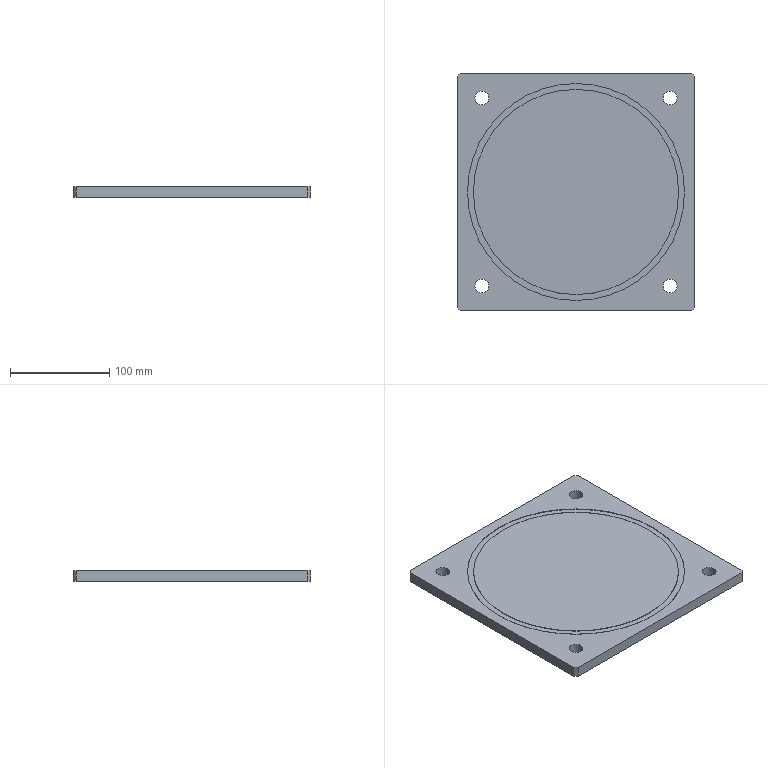Part | SolidWorks | features ICE 2, Chamfer 1, Extrusion 1 | 1 solid | 24 faces | box 240 x 240 x 11 mm | volume 624621 mm3 | cylinder 12 | plane 12 | commonest cylinder face diameters 14 x8 207 x2 219 x2
STEP:
#1=CARTESIAN_POINT('',(-88.,-95.,0.));
#2=VERTEX_POINT('',#1);
#3=CARTESIAN_POINT('',(-102.,-95.,0.));
#4=VERTEX_POINT('',#3);
#5=CARTESIAN_POINT('',(-95.,-95.,0.));
#6=DIRECTION('',(0.,0.,-1.));
#7=DIRECTION('',(-1.,0.,0.));
#8=AXIS2_PLACEMENT_3D('',#5,#6,#7);
#9=CIRCLE('',#8,7.);
#10=EDGE_CURVE('',#2,#4,#9,.T.);
#11=ORIENTED_EDGE('',*,*,#10,.T.);
#12=CARTESIAN_POINT('',(-102.,-95.,11.));
#13=VERTEX_POINT('',#12);
#14=CARTESIAN_POINT('',(-102.,-95.,-48.));
#15=DIRECTION('',(0.,0.,1.));
#16=VECTOR('',#15,1000.);
#17=LINE('',#14,#16);
#18=EDGE_CURVE('',#4,#13,#17,.T.);
#19=ORIENTED_EDGE('',*,*,#18,.T.);
#20=CARTESIAN_POINT('',(-88.,-95.,11.));
#21=VERTEX_POINT('',#20);
#22=CARTESIAN_POINT('',(-95.,-95.,11.));
#23=DIRECTION('',(0.,0.,1.));
#24=DIRECTION('',(1.,0.,0.));
#25=AXIS2_PLACEMENT_3D('',#22,#23,#24);
#26=CIRCLE('',#25,7.);
#27=EDGE_CURVE('',#13,#21,#26,.T.);
#28=ORIENTED_EDGE('',*,*,#27,.T.);
#29=CARTESIAN_POINT('',(-88.,-95.,-48.));
#30=DIRECTION('',(0.,0.,1.));
#31=VECTOR('',#30,1000.);
#32=LINE('',#29,#31);
#33=EDGE_CURVE('',#2,#21,#32,.T.);
#34=ORIENTED_EDGE('',*,*,#33,.F.);
#35=EDGE_LOOP('',(#11,#19,#28,#34));
#36=FACE_OUTER_BOUND('',#35,.T.);
#37=CARTESIAN_POINT('',(-95.,-95.,-48.));
#38=DIRECTION('',(0.,0.,1.));
#39=DIRECTION('',(1.,0.,0.));
#40=AXIS2_PLACEMENT_3D('',#37,#38,#39);
#41=CYLINDRICAL_SURFACE('',#40,7.);
#42=ADVANCED_FACE('',(#36),#41,.F.);
#43=CARTESIAN_POINT('',(102.,-95.,0.));
#44=VERTEX_POINT('',#43);
#45=CARTESIAN_POINT('',(88.,-95.,0.));
#46=VERTEX_POINT('',#45);
#47=CARTESIAN_POINT('',(95.,-95.,0.));
#48=DIRECTION('',(0.,0.,-1.));
#49=DIRECTION('',(-1.,0.,0.));
#50=AXIS2_PLACEMENT_3D('',#47,#48,#49);
#51=CIRCLE('',#50,7.);
#52=EDGE_CURVE('',#44,#46,#51,.T.);
#53=ORIENTED_EDGE('',*,*,#52,.T.);
#54=CARTESIAN_POINT('',(88.,-95.,11.));
#55=VERTEX_POINT('',#54);
#56=CARTESIAN_POINT('',(88.,-95.,-48.));
#57=DIRECTION('',(0.,0.,1.));
#58=VECTOR('',#57,1000.);
#59=LINE('',#56,#58);
#60=EDGE_CURVE('',#46,#55,#59,.T.);
#61=ORIENTED_EDGE('',*,*,#60,.T.);
#62=CARTESIAN_POINT('',(102.,-95.,11.));
#63=VERTEX_POINT('',#62);
#64=CARTESIAN_POINT('',(95.,-95.,11.));
#65=DIRECTION('',(0.,0.,1.));
#66=DIRECTION('',(1.,0.,0.));
#67=AXIS2_PLACEMENT_3D('',#64,#65,#66);
#68=CIRCLE('',#67,7.);
#69=EDGE_CURVE('',#55,#63,#68,.T.);
#70=ORIENTED_EDGE('',*,*,#69,.T.);
#71=CARTESIAN_POINT('',(102.,-95.,-48.));
#72=DIRECTION('',(0.,0.,1.));
#73=VECTOR('',#72,1000.);
#74=LINE('',#71,#73);
#75=EDGE_CURVE('',#44,#63,#74,.T.);
#76=ORIENTED_EDGE('',*,*,#75,.F.);
#77=EDGE_LOOP('',(#53,#61,#70,#76));
#78=FACE_OUTER_BOUND('',#77,.T.);
#79=CARTESIAN_POINT('',(95.,-95.,-48.));
#80=DIRECTION('',(0.,0.,1.));
#81=DIRECTION('',(1.,0.,0.));
#82=AXIS2_PLACEMENT_3D('',#79,#80,#81);
#83=CYLINDRICAL_SURFACE('',#82,7.);
#84=ADVANCED_FACE('',(#78),#83,.F.);
#85=CARTESIAN_POINT('',(102.,95.,0.));
#86=VERTEX_POINT('',#85);
#87=CARTESIAN_POINT('',(88.,95.,0.));
#88=VERTEX_POINT('',#87);
#89=CARTESIAN_POINT('',(95.,95.,0.));
#90=DIRECTION('',(0.,0.,-1.));
#91=DIRECTION('',(-1.,0.,0.));
#92=AXIS2_PLACEMENT_3D('',#89,#90,#91);
#93=CIRCLE('',#92,7.);
#94=EDGE_CURVE('',#86,#88,#93,.T.);
#95=ORIENTED_EDGE('',*,*,#94,.T.);
#96=CARTESIAN_POINT('',(88.,95.,11.));
#97=VERTEX_POINT('',#96);
#98=CARTESIAN_POINT('',(88.,95.,-48.));
#99=DIRECTION('',(0.,0.,1.));
#100=VECTOR('',#99,1000.);
#101=LINE('',#98,#100);
#102=EDGE_CURVE('',#88,#97,#101,.T.);
#103=ORIENTED_EDGE('',*,*,#102,.T.);
#104=CARTESIAN_POINT('',(102.,95.,11.));
#105=VERTEX_POINT('',#104);
#106=CARTESIAN_POINT('',(95.,95.,11.));
#107=DIRECTION('',(0.,0.,1.));
#108=DIRECTION('',(1.,0.,0.));
#109=AXIS2_PLACEMENT_3D('',#106,#107,#108);
#110=CIRCLE('',#109,7.);
#111=EDGE_CURVE('',#97,#105,#110,.T.);
#112=ORIENTED_EDGE('',*,*,#111,.T.);
#113=CARTESIAN_POINT('',(102.,95.,-48.));
#114=DIRECTION('',(0.,0.,1.));
#115=VECTOR('',#114,1000.);
#116=LINE('',#113,#115);
#117=EDGE_CURVE('',#86,#105,#116,.T.);
#118=ORIENTED_EDGE('',*,*,#117,.F.);
#119=EDGE_LOOP('',(#95,#103,#112,#118));
#120=FACE_OUTER_BOUND('',#119,.T.);
#121=CARTESIAN_POINT('',(95.,95.,-48.));
#122=DIRECTION('',(0.,0.,1.));
#123=DIRECTION('',(1.,0.,0.));
#124=AXIS2_PLACEMENT_3D('',#121,#122,#123);
#125=CYLINDRICAL_SURFACE('',#124,7.);
#126=ADVANCED_FACE('',(#120),#125,.F.);
#127=CARTESIAN_POINT('',(-88.,95.,0.));
#128=VERTEX_POINT('',#127);
#129=CARTESIAN_POINT('',(-102.,95.,0.));
#130=VERTEX_POINT('',#129);
#131=CARTESIAN_POINT('',(-95.,95.,0.));
#132=DIRECTION('',(0.,0.,-1.));
#133=DIRECTION('',(-1.,0.,0.));
#134=AXIS2_PLACEMENT_3D('',#131,#132,#133);
#135=CIRCLE('',#134,7.);
#136=EDGE_CURVE('',#128,#130,#135,.T.);
#137=ORIENTED_EDGE('',*,*,#136,.T.);
#138=CARTESIAN_POINT('',(-102.,95.,11.));
#139=VERTEX_POINT('',#138);
#140=CARTESIAN_POINT('',(-102.,95.,-48.));
#141=DIRECTION('',(0.,0.,1.));
#142=VECTOR('',#141,1000.);
#143=LINE('',#140,#142);
#144=EDGE_CURVE('',#130,#139,#143,.T.);
#145=ORIENTED_EDGE('',*,*,#144,.T.);
#146=CARTESIAN_POINT('',(-88.,95.,11.));
#147=VERTEX_POINT('',#146);
#148=CARTESIAN_POINT('',(-95.,95.,11.));
#149=DIRECTION('',(0.,0.,1.));
#150=DIRECTION('',(1.,0.,0.));
#151=AXIS2_PLACEMENT_3D('',#148,#149,#150);
#152=CIRCLE('',#151,7.);
#153=EDGE_CURVE('',#139,#147,#152,.T.);
#154=ORIENTED_EDGE('',*,*,#153,.T.);
#155=CARTESIAN_POINT('',(-88.,95.,-48.));
#156=DIRECTION('',(0.,0.,1.));
#157=VECTOR('',#156,1000.);
#158=LINE('',#155,#157);
#159=EDGE_CURVE('',#128,#147,#158,.T.);
#160=ORIENTED_EDGE('',*,*,#159,.F.);
#161=EDGE_LOOP('',(#137,#145,#154,#160));
#162=FACE_OUTER_BOUND('',#161,.T.);
#163=CARTESIAN_POINT('',(-95.,95.,-48.));
#164=DIRECTION('',(0.,0.,1.));
#165=DIRECTION('',(1.,0.,0.));
#166=AXIS2_PLACEMENT_3D('',#163,#164,#165);
#167=CYLINDRICAL_SURFACE('',#166,7.);
#168=ADVANCED_FACE('',(#162),#167,.F.);
#169=CARTESIAN_POINT('',(103.5,0.,10.5));
#170=VERTEX_POINT('',#169);
#171=CARTESIAN_POINT('',(-103.5,0.,10.5));
#172=VERTEX_POINT('',#171);
#173=CARTESIAN_POINT('',(0.,0.,10.5));
#174=DIRECTION('',(0.,0.,1.));
#175=DIRECTION('',(1.,0.,0.));
#176=AXIS2_PLACEMENT_3D('',#173,#174,#175);
#177=CIRCLE('',#176,103.5);
#178=EDGE_CURVE('',#170,#172,#177,.T.);
#179=ORIENTED_EDGE('',*,*,#178,.T.);
#180=CARTESIAN_POINT('',(-103.5,0.,11.));
#181=VERTEX_POINT('',#180);
#182=CARTESIAN_POINT('',(-103.5,0.,10.5));
#183=DIRECTION('',(0.,0.,1.));
#184=VECTOR('',#183,1000.);
#185=LINE('',#182,#184);
#186=EDGE_CURVE('',#172,#181,#185,.T.);
#187=ORIENTED_EDGE('',*,*,#186,.T.);
#188=CARTESIAN_POINT('',(103.5,0.,11.));
#189=VERTEX_POINT('',#188);
#190=CARTESIAN_POINT('',(0.,0.,11.));
#191=DIRECTION('',(0.,0.,1.));
#192=DIRECTION('',(1.,0.,0.));
#193=AXIS2_PLACEMENT_3D('',#190,#191,#192);
#194=CIRCLE('',#193,103.5);
#195=EDGE_CURVE('',#189,#181,#194,.T.);
#196=ORIENTED_EDGE('',*,*,#195,.F.);
#197=CARTESIAN_POINT('',(103.5,0.,10.5));
#198=DIRECTION('',(0.,0.,1.));
#199=VECTOR('',#198,1000.);
#200=LINE('',#197,#199);
#201=EDGE_CURVE('',#170,#189,#200,.T.);
#202=ORIENTED_EDGE('',*,*,#201,.F.);
#203=EDGE_LOOP('',(#179,#187,#196,#202));
#204=FACE_OUTER_BOUND('',#203,.T.);
#205=CARTESIAN_POINT('',(0.,0.,10.5));
#206=DIRECTION('',(0.,0.,1.));
#207=DIRECTION('',(1.,0.,0.));
#208=AXIS2_PLACEMENT_3D('',#205,#206,#207);
#209=CYLINDRICAL_SURFACE('',#208,103.5);
#210=ADVANCED_FACE('',(#204),#209,.T.);
#211=CARTESIAN_POINT('',(-109.5,0.,10.5));
#212=VERTEX_POINT('',#211);
#213=CARTESIAN_POINT('',(109.5,0.,10.5));
#214=VERTEX_POINT('',#213);
#215=CARTESIAN_POINT('',(0.,0.,10.5));
#216=DIRECTION('',(0.,0.,1.));
#217=DIRECTION('',(1.,0.,0.));
#218=AXIS2_PLACEMENT_3D('',#215,#216,#217);
#219=CIRCLE('',#218,109.5);
#220=EDGE_CURVE('',#212,#214,#219,.T.);
#221=ORIENTED_EDGE('',*,*,#220,.F.);
#222=CARTESIAN_POINT('',(-109.5,0.,11.));
#223=VERTEX_POINT('',#222);
#224=CARTESIAN_POINT('',(-109.5,0.,10.5));
#225=DIRECTION('',(0.,0.,1.));
#226=VECTOR('',#225,1000.);
#227=LINE('',#224,#226);
#228=EDGE_CURVE('',#212,#223,#227,.T.);
#229=ORIENTED_EDGE('',*,*,#228,.T.);
#230=CARTESIAN_POINT('',(109.5,0.,11.));
#231=VERTEX_POINT('',#230);
#232=CARTESIAN_POINT('',(0.,0.,11.));
#233=DIRECTION('',(0.,0.,1.));
#234=DIRECTION('',(1.,0.,0.));
#235=AXIS2_PLACEMENT_3D('',#232,#233,#234);
#236=CIRCLE('',#235,109.5);
#237=EDGE_CURVE('',#223,#231,#236,.T.);
#238=ORIENTED_EDGE('',*,*,#237,.T.);
#239=CARTESIAN_POINT('',(109.5,0.,10.5));
#240=DIRECTION('',(0.,0.,1.));
#241=VECTOR('',#240,1000.);
#242=LINE('',#239,#241);
#243=EDGE_CURVE('',#214,#231,#242,.T.);
#244=ORIENTED_EDGE('',*,*,#243,.F.);
#245=EDGE_LOOP('',(#221,#229,#238,#244));
#246=FACE_OUTER_BOUND('',#245,.T.);
#247=CARTESIAN_POINT('',(0.,0.,10.5));
#248=DIRECTION('',(0.,0.,1.));
#249=DIRECTION('',(1.,0.,0.));
#250=AXIS2_PLACEMENT_3D('',#247,#248,#249);
#251=CYLINDRICAL_SURFACE('',#250,109.5);
#252=ADVANCED_FACE('',(#246),#251,.F.);
#253=CARTESIAN_POINT('',(-120.,117.,0.));
#254=VERTEX_POINT('',#253);
#255=CARTESIAN_POINT('',(-120.,-117.,0.));
#256=VERTEX_POINT('',#255);
#257=CARTESIAN_POINT('',(-120.,120.,0.));
#258=DIRECTION('',(0.,-1.,0.));
#259=VECTOR('',#258,1000.);
#260=LINE('',#257,#259);
#261=EDGE_CURVE('',#254,#256,#260,.T.);
#262=ORIENTED_EDGE('',*,*,#261,.T.);
#263=CARTESIAN_POINT('',(-120.,-117.,11.));
#264=VERTEX_POINT('',#263);
#265=CARTESIAN_POINT('',(-120.,-117.,11.));
#266=DIRECTION('',(0.,0.,1.));
#267=VECTOR('',#266,1000.);
#268=LINE('',#265,#267);
#269=EDGE_CURVE('',#256,#264,#268,.T.);
#270=ORIENTED_EDGE('',*,*,#269,.T.);
#271=CARTESIAN_POINT('',(-120.,117.,11.));
#272=VERTEX_POINT('',#271);
#273=CARTESIAN_POINT('',(-120.,120.,11.));
#274=DIRECTION('',(0.,-1.,0.));
#275=VECTOR('',#274,1000.);
#276=LINE('',#273,#275);
#277=EDGE_CURVE('',#272,#264,#276,.T.);
#278=ORIENTED_EDGE('',*,*,#277,.F.);
#279=CARTESIAN_POINT('',(-120.,117.,11.));
#280=DIRECTION('',(0.,0.,-1.));
#281=VECTOR('',#280,1000.);
#282=LINE('',#279,#281);
#283=EDGE_CURVE('',#272,#254,#282,.T.);
#284=ORIENTED_EDGE('',*,*,#283,.T.);
#285=EDGE_LOOP('',(#262,#270,#278,#284));
#286=FACE_OUTER_BOUND('',#285,.T.);
#287=CARTESIAN_POINT('',(-120.,120.,11.));
#288=DIRECTION('',(1.,0.,0.));
#289=DIRECTION('',(0.,1.,0.));
#290=AXIS2_PLACEMENT_3D('',#287,#288,#289);
#291=PLANE('',#290);
#292=ADVANCED_FACE('',(#286),#291,.F.);
#293=CARTESIAN_POINT('',(-117.,-120.,11.));
#294=VERTEX_POINT('',#293);
#295=CARTESIAN_POINT('',(117.,-120.,11.));
#296=VERTEX_POINT('',#295);
#297=CARTESIAN_POINT('',(120.,-120.,11.));
#298=DIRECTION('',(1.,0.,0.));
#299=VECTOR('',#298,1000.);
#300=LINE('',#297,#299);
#301=EDGE_CURVE('',#294,#296,#300,.T.);
#302=ORIENTED_EDGE('',*,*,#301,.F.);
#303=CARTESIAN_POINT('',(-117.,-120.,0.));
#304=VERTEX_POINT('',#303);
#305=CARTESIAN_POINT('',(-117.,-120.,11.));
#306=DIRECTION('',(0.,0.,-1.));
#307=VECTOR('',#306,1000.);
#308=LINE('',#305,#307);
#309=EDGE_CURVE('',#294,#304,#308,.T.);
#310=ORIENTED_EDGE('',*,*,#309,.T.);
#311=CARTESIAN_POINT('',(117.,-120.,0.));
#312=VERTEX_POINT('',#311);
#313=CARTESIAN_POINT('',(120.,-120.,0.));
#314=DIRECTION('',(1.,0.,0.));
#315=VECTOR('',#314,1000.);
#316=LINE('',#313,#315);
#317=EDGE_CURVE('',#304,#312,#316,.T.);
#318=ORIENTED_EDGE('',*,*,#317,.T.);
#319=CARTESIAN_POINT('',(117.,-120.,11.));
#320=DIRECTION('',(0.,0.,1.));
#321=VECTOR('',#320,1000.);
#322=LINE('',#319,#321);
#323=EDGE_CURVE('',#312,#296,#322,.T.);
#324=ORIENTED_EDGE('',*,*,#323,.T.);
#325=EDGE_LOOP('',(#302,#310,#318,#324));
#326=FACE_OUTER_BOUND('',#325,.T.);
#327=CARTESIAN_POINT('',(120.,-120.,11.));
#328=DIRECTION('',(0.,1.,0.));
#329=DIRECTION('',(-1.,0.,0.));
#330=AXIS2_PLACEMENT_3D('',#327,#328,#329);
#331=PLANE('',#330);
#332=ADVANCED_FACE('',(#326),#331,.F.);
#333=CARTESIAN_POINT('',(120.,-117.,11.));
#334=VERTEX_POINT('',#333);
#335=CARTESIAN_POINT('',(120.,117.,11.));
#336=VERTEX_POINT('',#335);
#337=CARTESIAN_POINT('',(120.,120.,11.));
#338=DIRECTION('',(0.,1.,0.));
#339=VECTOR('',#338,1000.);
#340=LINE('',#337,#339);
#341=EDGE_CURVE('',#334,#336,#340,.T.);
#342=ORIENTED_EDGE('',*,*,#341,.F.);
#343=CARTESIAN_POINT('',(120.,-117.,0.));
#344=VERTEX_POINT('',#343);
#345=CARTESIAN_POINT('',(120.,-117.,11.));
#346=DIRECTION('',(0.,0.,-1.));
#347=VECTOR('',#346,1000.);
#348=LINE('',#345,#347);
#349=EDGE_CURVE('',#334,#344,#348,.T.);
#350=ORIENTED_EDGE('',*,*,#349,.T.);
#351=CARTESIAN_POINT('',(120.,117.,0.));
#352=VERTEX_POINT('',#351);
#353=CARTESIAN_POINT('',(120.,120.,0.));
#354=DIRECTION('',(0.,1.,0.));
#355=VECTOR('',#354,1000.);
#356=LINE('',#353,#355);
#357=EDGE_CURVE('',#344,#352,#356,.T.);
#358=ORIENTED_EDGE('',*,*,#357,.T.);
#359=CARTESIAN_POINT('',(120.,117.,11.));
#360=DIRECTION('',(0.,0.,1.));
#361=VECTOR('',#360,1000.);
#362=LINE('',#359,#361);
#363=EDGE_CURVE('',#352,#336,#362,.T.);
#364=ORIENTED_EDGE('',*,*,#363,.T.);
#365=EDGE_LOOP('',(#342,#350,#358,#364));
#366=FACE_OUTER_BOUND('',#365,.T.);
#367=CARTESIAN_POINT('',(120.,120.,11.));
#368=DIRECTION('',(-1.,0.,0.));
#369=DIRECTION('',(0.,-1.,0.));
#370=AXIS2_PLACEMENT_3D('',#367,#368,#369);
#371=PLANE('',#370);
#372=ADVANCED_FACE('',(#366),#371,.F.);
#373=CARTESIAN_POINT('',(117.,120.,11.));
#374=VERTEX_POINT('',#373);
#375=CARTESIAN_POINT('',(-117.,120.,11.));
#376=VERTEX_POINT('',#375);
#377=CARTESIAN_POINT('',(120.,120.,11.));
#378=DIRECTION('',(-1.,0.,0.));
#379=VECTOR('',#378,1000.);
#380=LINE('',#377,#379);
#381=EDGE_CURVE('',#374,#376,#380,.T.);
#382=ORIENTED_EDGE('',*,*,#381,.F.);
#383=CARTESIAN_POINT('',(117.,120.,0.));
#384=VERTEX_POINT('',#383);
#385=CARTESIAN_POINT('',(117.,120.,11.));
#386=DIRECTION('',(0.,0.,-1.));
#387=VECTOR('',#386,1000.);
#388=LINE('',#385,#387);
#389=EDGE_CURVE('',#374,#384,#388,.T.);
#390=ORIENTED_EDGE('',*,*,#389,.T.);
#391=CARTESIAN_POINT('',(-117.,120.,0.));
#392=VERTEX_POINT('',#391);
#393=CARTESIAN_POINT('',(120.,120.,0.));
#394=DIRECTION('',(-1.,0.,0.));
#395=VECTOR('',#394,1000.);
#396=LINE('',#393,#395);
#397=EDGE_CURVE('',#384,#392,#396,.T.);
#398=ORIENTED_EDGE('',*,*,#397,.T.);
#399=CARTESIAN_POINT('',(-117.,120.,11.));
#400=DIRECTION('',(0.,0.,1.));
#401=VECTOR('',#400,1000.);
#402=LINE('',#399,#401);
#403=EDGE_CURVE('',#392,#376,#402,.T.);
#404=ORIENTED_EDGE('',*,*,#403,.T.);
#405=EDGE_LOOP('',(#382,#390,#398,#404));
#406=FACE_OUTER_BOUND('',#405,.T.);
#407=CARTESIAN_POINT('',(120.,120.,11.));
#408=DIRECTION('',(0.,-1.,0.));
#409=DIRECTION('',(1.,0.,0.));
#410=AXIS2_PLACEMENT_3D('',#407,#408,#409);
#411=PLANE('',#410);
#412=ADVANCED_FACE('',(#406),#411,.F.);
#413=CARTESIAN_POINT('',(-95.,-95.,11.));
#414=DIRECTION('',(0.,0.,1.));
#415=DIRECTION('',(1.,0.,0.));
#416=AXIS2_PLACEMENT_3D('',#413,#414,#415);
#417=CIRCLE('',#416,7.);
#418=EDGE_CURVE('',#21,#13,#417,.T.);
#419=ORIENTED_EDGE('',*,*,#418,.F.);
#420=ORIENTED_EDGE('',*,*,#27,.F.);
#421=EDGE_LOOP('',(#419,#420));
#422=FACE_BOUND('',#421,.T.);
#423=CARTESIAN_POINT('',(95.,-95.,11.));
#424=DIRECTION('',(0.,0.,1.));
#425=DIRECTION('',(1.,0.,0.));
#426=AXIS2_PLACEMENT_3D('',#423,#424,#425);
#427=CIRCLE('',#426,7.);
#428=EDGE_CURVE('',#63,#55,#427,.T.);
#429=ORIENTED_EDGE('',*,*,#428,.F.);
#430=ORIENTED_EDGE('',*,*,#69,.F.);
#431=EDGE_LOOP('',(#429,#430));
#432=FACE_BOUND('',#431,.T.);
#433=CARTESIAN_POINT('',(95.,95.,11.));
#434=DIRECTION('',(0.,0.,1.));
#435=DIRECTION('',(1.,0.,0.));
#436=AXIS2_PLACEMENT_3D('',#433,#434,#435);
#437=CIRCLE('',#436,7.);
#438=EDGE_CURVE('',#105,#97,#437,.T.);
#439=ORIENTED_EDGE('',*,*,#438,.F.);
#440=ORIENTED_EDGE('',*,*,#111,.F.);
#441=EDGE_LOOP('',(#439,#440));
#442=FACE_BOUND('',#441,.T.);
#443=CARTESIAN_POINT('',(-95.,95.,11.));
#444=DIRECTION('',(0.,0.,1.));
#445=DIRECTION('',(1.,0.,0.));
#446=AXIS2_PLACEMENT_3D('',#443,#444,#445);
#447=CIRCLE('',#446,7.);
#448=EDGE_CURVE('',#147,#139,#447,.T.);
#449=ORIENTED_EDGE('',*,*,#448,.F.);
#450=ORIENTED_EDGE('',*,*,#153,.F.);
#451=EDGE_LOOP('',(#449,#450));
#452=FACE_BOUND('',#451,.T.);
#453=CARTESIAN_POINT('',(0.,0.,11.));
#454=DIRECTION('',(0.,0.,1.));
#455=DIRECTION('',(1.,0.,0.));
#456=AXIS2_PLACEMENT_3D('',#453,#454,#455);
#457=CIRCLE('',#456,109.5);
#458=EDGE_CURVE('',#231,#223,#457,.T.);
#459=ORIENTED_EDGE('',*,*,#458,.F.);
#460=ORIENTED_EDGE('',*,*,#237,.F.);
#461=EDGE_LOOP('',(#459,#460));
#462=FACE_BOUND('',#461,.T.);
#463=ORIENTED_EDGE('',*,*,#277,.T.);
#464=CARTESIAN_POINT('',(-117.,-120.,11.));
#465=DIRECTION('',(0.7071,-0.7071,0.));
#466=VECTOR('',#465,1000.);
#467=LINE('',#464,#466);
#468=EDGE_CURVE('',#264,#294,#467,.T.);
#469=ORIENTED_EDGE('',*,*,#468,.T.);
#470=ORIENTED_EDGE('',*,*,#301,.T.);
#471=CARTESIAN_POINT('',(120.,-117.,11.));
#472=DIRECTION('',(0.7071,0.7071,0.));
#473=VECTOR('',#472,1000.);
#474=LINE('',#471,#473);
#475=EDGE_CURVE('',#296,#334,#474,.T.);
#476=ORIENTED_EDGE('',*,*,#475,.T.);
#477=ORIENTED_EDGE('',*,*,#341,.T.);
#478=CARTESIAN_POINT('',(117.,120.,11.));
#479=DIRECTION('',(-0.7071,0.7071,0.));
#480=VECTOR('',#479,1000.);
#481=LINE('',#478,#480);
#482=EDGE_CURVE('',#336,#374,#481,.T.);
#483=ORIENTED_EDGE('',*,*,#482,.T.);
#484=ORIENTED_EDGE('',*,*,#381,.T.);
#485=CARTESIAN_POINT('',(-120.,117.,11.));
#486=DIRECTION('',(-0.7071,-0.7071,0.));
#487=VECTOR('',#486,1000.);
#488=LINE('',#485,#487);
#489=EDGE_CURVE('',#376,#272,#488,.T.);
#490=ORIENTED_EDGE('',*,*,#489,.T.);
#491=EDGE_LOOP('',(#463,#469,#470,#476,#477,#483,#484,#490));
#492=FACE_OUTER_BOUND('',#491,.T.);
#493=CARTESIAN_POINT('',(0.,0.,11.));
#494=DIRECTION('',(0.,0.,-1.));
#495=DIRECTION('',(-1.,0.,0.));
#496=AXIS2_PLACEMENT_3D('',#493,#494,#495);
#497=PLANE('',#496);
#498=ADVANCED_FACE('',(#422,#432,#442,#452,#462,#492),#497,.F.);
#499=ORIENTED_EDGE('',*,*,#10,.F.);
#500=CARTESIAN_POINT('',(-95.,-95.,0.));
#501=DIRECTION('',(0.,0.,-1.));
#502=DIRECTION('',(-1.,0.,0.));
#503=AXIS2_PLACEMENT_3D('',#500,#501,#502);
#504=CIRCLE('',#503,7.);
#505=EDGE_CURVE('',#4,#2,#504,.T.);
#506=ORIENTED_EDGE('',*,*,#505,.F.);
#507=EDGE_LOOP('',(#499,#506));
#508=FACE_BOUND('',#507,.T.);
#509=ORIENTED_EDGE('',*,*,#52,.F.);
#510=CARTESIAN_POINT('',(95.,-95.,0.));
#511=DIRECTION('',(0.,0.,-1.));
#512=DIRECTION('',(-1.,0.,0.));
#513=AXIS2_PLACEMENT_3D('',#510,#511,#512);
#514=CIRCLE('',#513,7.);
#515=EDGE_CURVE('',#46,#44,#514,.T.);
#516=ORIENTED_EDGE('',*,*,#515,.F.);
#517=EDGE_LOOP('',(#509,#516));
#518=FACE_BOUND('',#517,.T.);
#519=ORIENTED_EDGE('',*,*,#94,.F.);
#520=CARTESIAN_POINT('',(95.,95.,0.));
#521=DIRECTION('',(0.,0.,-1.));
#522=DIRECTION('',(-1.,0.,0.));
#523=AXIS2_PLACEMENT_3D('',#520,#521,#522);
#524=CIRCLE('',#523,7.);
#525=EDGE_CURVE('',#88,#86,#524,.T.);
#526=ORIENTED_EDGE('',*,*,#525,.F.);
#527=EDGE_LOOP('',(#519,#526));
#528=FACE_BOUND('',#527,.T.);
#529=ORIENTED_EDGE('',*,*,#136,.F.);
#530=CARTESIAN_POINT('',(-95.,95.,0.));
#531=DIRECTION('',(0.,0.,-1.));
#532=DIRECTION('',(-1.,0.,0.));
#533=AXIS2_PLACEMENT_3D('',#530,#531,#532);
#534=CIRCLE('',#533,7.);
#535=EDGE_CURVE('',#130,#128,#534,.T.);
#536=ORIENTED_EDGE('',*,*,#535,.F.);
#537=EDGE_LOOP('',(#529,#536));
#538=FACE_BOUND('',#537,.T.);
#539=ORIENTED_EDGE('',*,*,#317,.F.);
#540=CARTESIAN_POINT('',(-118.5,-118.5,0.));
#541=DIRECTION('',(-0.7071,0.7071,0.));
#542=VECTOR('',#541,1000.);
#543=LINE('',#540,#542);
#544=EDGE_CURVE('',#304,#256,#543,.T.);
#545=ORIENTED_EDGE('',*,*,#544,.T.);
#546=ORIENTED_EDGE('',*,*,#261,.F.);
#547=CARTESIAN_POINT('',(-118.5,118.5,0.));
#548=DIRECTION('',(0.7071,0.7071,0.));
#549=VECTOR('',#548,1000.);
#550=LINE('',#547,#549);
#551=EDGE_CURVE('',#254,#392,#550,.T.);
#552=ORIENTED_EDGE('',*,*,#551,.T.);
#553=ORIENTED_EDGE('',*,*,#397,.F.);
#554=CARTESIAN_POINT('',(118.5,118.5,0.));
#555=DIRECTION('',(0.7071,-0.7071,0.));
#556=VECTOR('',#555,1000.);
#557=LINE('',#554,#556);
#558=EDGE_CURVE('',#384,#352,#557,.T.);
#559=ORIENTED_EDGE('',*,*,#558,.T.);
#560=ORIENTED_EDGE('',*,*,#357,.F.);
#561=CARTESIAN_POINT('',(118.5,-118.5,0.));
#562=DIRECTION('',(-0.7071,-0.7071,0.));
#563=VECTOR('',#562,1000.);
#564=LINE('',#561,#563);
#565=EDGE_CURVE('',#344,#312,#564,.T.);
#566=ORIENTED_EDGE('',*,*,#565,.T.);
#567=EDGE_LOOP('',(#539,#545,#546,#552,#553,#559,#560,#566));
#568=FACE_OUTER_BOUND('',#567,.T.);
#569=CARTESIAN_POINT('',(0.,0.,0.));
#570=DIRECTION('',(0.,0.,-1.));
#571=DIRECTION('',(-1.,0.,0.));
#572=AXIS2_PLACEMENT_3D('',#569,#570,#571);
#573=PLANE('',#572);
#574=ADVANCED_FACE('',(#508,#518,#528,#538,#568),#573,.T.);
#575=ORIENTED_EDGE('',*,*,#228,.F.);
#576=CARTESIAN_POINT('',(0.,0.,10.5));
#577=DIRECTION('',(0.,0.,1.));
#578=DIRECTION('',(1.,0.,0.));
#579=AXIS2_PLACEMENT_3D('',#576,#577,#578);
#580=CIRCLE('',#579,109.5);
#581=EDGE_CURVE('',#214,#212,#580,.T.);
#582=ORIENTED_EDGE('',*,*,#581,.F.);
#583=ORIENTED_EDGE('',*,*,#243,.T.);
#584=ORIENTED_EDGE('',*,*,#458,.T.);
#585=EDGE_LOOP('',(#575,#582,#583,#584));
#586=FACE_OUTER_BOUND('',#585,.T.);
#587=CARTESIAN_POINT('',(0.,0.,10.5));
#588=DIRECTION('',(0.,0.,1.));
#589=DIRECTION('',(1.,0.,0.));
#590=AXIS2_PLACEMENT_3D('',#587,#588,#589);
#591=CYLINDRICAL_SURFACE('',#590,109.5);
#592=ADVANCED_FACE('',(#586),#591,.F.);
#593=ORIENTED_EDGE('',*,*,#178,.F.);
#594=CARTESIAN_POINT('',(0.,0.,10.5));
#595=DIRECTION('',(0.,0.,1.));
#596=DIRECTION('',(1.,0.,0.));
#597=AXIS2_PLACEMENT_3D('',#594,#595,#596);
#598=CIRCLE('',#597,103.5);
#599=EDGE_CURVE('',#172,#170,#598,.T.);
#600=ORIENTED_EDGE('',*,*,#599,.F.);
#601=EDGE_LOOP('',(#593,#600));
#602=FACE_BOUND('',#601,.T.);
#603=ORIENTED_EDGE('',*,*,#581,.T.);
#604=ORIENTED_EDGE('',*,*,#220,.T.);
#605=EDGE_LOOP('',(#603,#604));
#606=FACE_OUTER_BOUND('',#605,.T.);
#607=CARTESIAN_POINT('',(0.,0.,10.5));
#608=DIRECTION('',(0.,0.,1.));
#609=DIRECTION('',(1.,0.,0.));
#610=AXIS2_PLACEMENT_3D('',#607,#608,#609);
#611=PLANE('',#610);
#612=ADVANCED_FACE('',(#602,#606),#611,.T.);
#613=ORIENTED_EDGE('',*,*,#186,.F.);
#614=ORIENTED_EDGE('',*,*,#599,.T.);
#615=ORIENTED_EDGE('',*,*,#201,.T.);
#616=CARTESIAN_POINT('',(0.,0.,11.));
#617=DIRECTION('',(0.,0.,1.));
#618=DIRECTION('',(1.,0.,0.));
#619=AXIS2_PLACEMENT_3D('',#616,#617,#618);
#620=CIRCLE('',#619,103.5);
#621=EDGE_CURVE('',#181,#189,#620,.T.);
#622=ORIENTED_EDGE('',*,*,#621,.F.);
#623=EDGE_LOOP('',(#613,#614,#615,#622));
#624=FACE_OUTER_BOUND('',#623,.T.);
#625=CARTESIAN_POINT('',(0.,0.,10.5));
#626=DIRECTION('',(0.,0.,1.));
#627=DIRECTION('',(1.,0.,0.));
#628=AXIS2_PLACEMENT_3D('',#625,#626,#627);
#629=CYLINDRICAL_SURFACE('',#628,103.5);
#630=ADVANCED_FACE('',(#624),#629,.T.);
#631=ORIENTED_EDGE('',*,*,#195,.T.);
#632=ORIENTED_EDGE('',*,*,#621,.T.);
#633=EDGE_LOOP('',(#631,#632));
#634=FACE_OUTER_BOUND('',#633,.T.);
#635=CARTESIAN_POINT('',(0.,0.,11.));
#636=DIRECTION('',(0.,0.,-1.));
#637=DIRECTION('',(-1.,0.,0.));
#638=AXIS2_PLACEMENT_3D('',#635,#636,#637);
#639=PLANE('',#638);
#640=ADVANCED_FACE('',(#634),#639,.F.);
#641=ORIENTED_EDGE('',*,*,#144,.F.);
#642=ORIENTED_EDGE('',*,*,#535,.T.);
#643=ORIENTED_EDGE('',*,*,#159,.T.);
#644=ORIENTED_EDGE('',*,*,#448,.T.);
#645=EDGE_LOOP('',(#641,#642,#643,#644));
#646=FACE_OUTER_BOUND('',#645,.T.);
#647=CARTESIAN_POINT('',(-95.,95.,-48.));
#648=DIRECTION('',(0.,0.,1.));
#649=DIRECTION('',(1.,0.,0.));
#650=AXIS2_PLACEMENT_3D('',#647,#648,#649);
#651=CYLINDRICAL_SURFACE('',#650,7.);
#652=ADVANCED_FACE('',(#646),#651,.F.);
#653=ORIENTED_EDGE('',*,*,#102,.F.);
#654=ORIENTED_EDGE('',*,*,#525,.T.);
#655=ORIENTED_EDGE('',*,*,#117,.T.);
#656=ORIENTED_EDGE('',*,*,#438,.T.);
#657=EDGE_LOOP('',(#653,#654,#655,#656));
#658=FACE_OUTER_BOUND('',#657,.T.);
#659=CARTESIAN_POINT('',(95.,95.,-48.));
#660=DIRECTION('',(0.,0.,1.));
#661=DIRECTION('',(1.,0.,0.));
#662=AXIS2_PLACEMENT_3D('',#659,#660,#661);
#663=CYLINDRICAL_SURFACE('',#662,7.);
#664=ADVANCED_FACE('',(#658),#663,.F.);
#665=ORIENTED_EDGE('',*,*,#60,.F.);
#666=ORIENTED_EDGE('',*,*,#515,.T.);
#667=ORIENTED_EDGE('',*,*,#75,.T.);
#668=ORIENTED_EDGE('',*,*,#428,.T.);
#669=EDGE_LOOP('',(#665,#666,#667,#668));
#670=FACE_OUTER_BOUND('',#669,.T.);
#671=CARTESIAN_POINT('',(95.,-95.,-48.));
#672=DIRECTION('',(0.,0.,1.));
#673=DIRECTION('',(1.,0.,0.));
#674=AXIS2_PLACEMENT_3D('',#671,#672,#673);
#675=CYLINDRICAL_SURFACE('',#674,7.);
#676=ADVANCED_FACE('',(#670),#675,.F.);
#677=ORIENTED_EDGE('',*,*,#18,.F.);
#678=ORIENTED_EDGE('',*,*,#505,.T.);
#679=ORIENTED_EDGE('',*,*,#33,.T.);
#680=ORIENTED_EDGE('',*,*,#418,.T.);
#681=EDGE_LOOP('',(#677,#678,#679,#680));
#682=FACE_OUTER_BOUND('',#681,.T.);
#683=CARTESIAN_POINT('',(-95.,-95.,-48.));
#684=DIRECTION('',(0.,0.,1.));
#685=DIRECTION('',(1.,0.,0.));
#686=AXIS2_PLACEMENT_3D('',#683,#684,#685);
#687=CYLINDRICAL_SURFACE('',#686,7.);
#688=ADVANCED_FACE('',(#682),#687,.F.);
#689=ORIENTED_EDGE('',*,*,#468,.F.);
#690=ORIENTED_EDGE('',*,*,#269,.F.);
#691=ORIENTED_EDGE('',*,*,#544,.F.);
#692=ORIENTED_EDGE('',*,*,#309,.F.);
#693=EDGE_LOOP('',(#689,#690,#691,#692));
#694=FACE_OUTER_BOUND('',#693,.T.);
#695=CARTESIAN_POINT('',(-117.,-120.,11.));
#696=DIRECTION('',(0.7071,0.7071,0.));
#697=DIRECTION('',(0.,0.,-1.));
#698=AXIS2_PLACEMENT_3D('',#695,#696,#697);
#699=PLANE('',#698);
#700=ADVANCED_FACE('',(#694),#699,.F.);
#701=ORIENTED_EDGE('',*,*,#475,.F.);
#702=ORIENTED_EDGE('',*,*,#323,.F.);
#703=ORIENTED_EDGE('',*,*,#565,.F.);
#704=ORIENTED_EDGE('',*,*,#349,.F.);
#705=EDGE_LOOP('',(#701,#702,#703,#704));
#706=FACE_OUTER_BOUND('',#705,.T.);
#707=CARTESIAN_POINT('',(120.,-117.,11.));
#708=DIRECTION('',(-0.7071,0.7071,0.));
#709=DIRECTION('',(0.,0.,-1.));
#710=AXIS2_PLACEMENT_3D('',#707,#708,#709);
#711=PLANE('',#710);
#712=ADVANCED_FACE('',(#706),#711,.F.);
#713=ORIENTED_EDGE('',*,*,#482,.F.);
#714=ORIENTED_EDGE('',*,*,#363,.F.);
#715=ORIENTED_EDGE('',*,*,#558,.F.);
#716=ORIENTED_EDGE('',*,*,#389,.F.);
#717=EDGE_LOOP('',(#713,#714,#715,#716));
#718=FACE_OUTER_BOUND('',#717,.T.);
#719=CARTESIAN_POINT('',(117.,120.,11.));
#720=DIRECTION('',(-0.7071,-0.7071,0.));
#721=DIRECTION('',(0.,0.,-1.));
#722=AXIS2_PLACEMENT_3D('',#719,#720,#721);
#723=PLANE('',#722);
#724=ADVANCED_FACE('',(#718),#723,.F.);
#725=ORIENTED_EDGE('',*,*,#489,.F.);
#726=ORIENTED_EDGE('',*,*,#403,.F.);
#727=ORIENTED_EDGE('',*,*,#551,.F.);
#728=ORIENTED_EDGE('',*,*,#283,.F.);
#729=EDGE_LOOP('',(#725,#726,#727,#728));
#730=FACE_OUTER_BOUND('',#729,.T.);
#731=CARTESIAN_POINT('',(-120.,117.,11.));
#732=DIRECTION('',(0.7071,-0.7071,0.));
#733=DIRECTION('',(0.,0.,-1.));
#734=AXIS2_PLACEMENT_3D('',#731,#732,#733);
#735=PLANE('',#734);
#736=ADVANCED_FACE('',(#730),#735,.F.);
#737=CLOSED_SHELL('',(#42,#84,#126,#168,#210,#252,#292,#332,#372,#412,#498,#574,#592,#612,#630,#640,#652,#664,#676,#688,#700,#712,#724,#736));
#738=MANIFOLD_SOLID_BREP('',#737);
#739=CARTESIAN_POINT('',(0.,0.,0.));
#740=DIRECTION('',(0.,0.,1.));
#741=DIRECTION('',(1.,0.,0.));
#742=AXIS2_PLACEMENT_3D('',#739,#740,#741);
#743=(LENGTH_UNIT()NAMED_UNIT(*)SI_UNIT(.MILLI.,.METRE.));
#744=UNCERTAINTY_MEASURE_WITH_UNIT(LENGTH_MEASURE(0.00001),#743,'','');
#745=(NAMED_UNIT(*)PLANE_ANGLE_UNIT()SI_UNIT($,.RADIAN.));
#746=(NAMED_UNIT(*)SI_UNIT($,.STERADIAN.)SOLID_ANGLE_UNIT());
#747=(GEOMETRIC_REPRESENTATION_CONTEXT(3)GLOBAL_UNCERTAINTY_ASSIGNED_CONTEXT((#744))GLOBAL_UNIT_ASSIGNED_CONTEXT((#743,#745,#746))REPRESENTATION_CONTEXT('',''));
#748=ADVANCED_BREP_SHAPE_REPRESENTATION('',(#738,#742),#747);